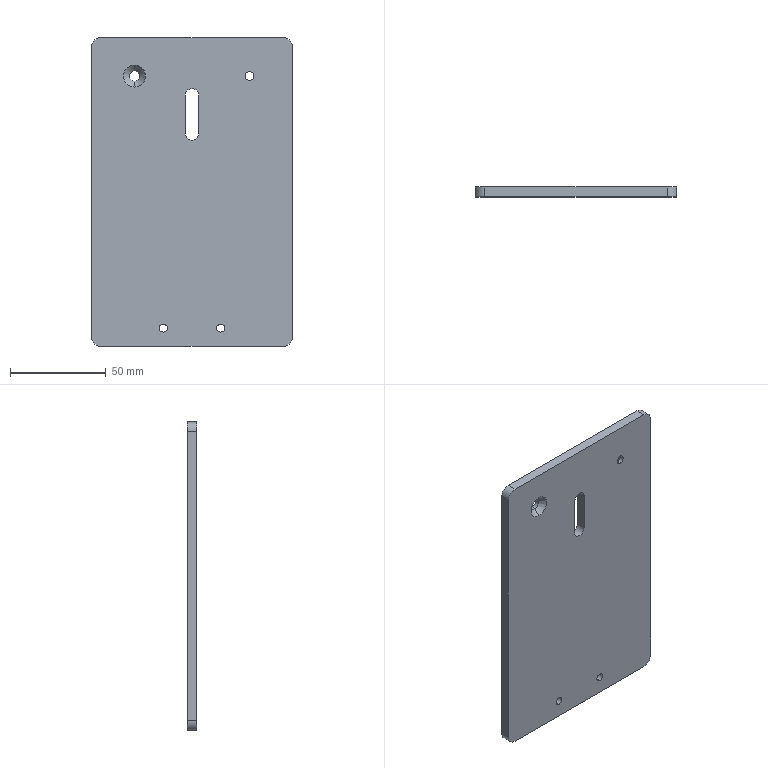Part | STEP file | H_ND24021-01-JG-108-SL | 1 solid | 27 faces | box 105 x 5 x 161 mm | volume 82990 mm3 | cylinder 15 | plane 8 | cone 4 | commonest cylinder face diameters 4.2 x4 10 x4 7 x3 4.5 x2 5.5 x2